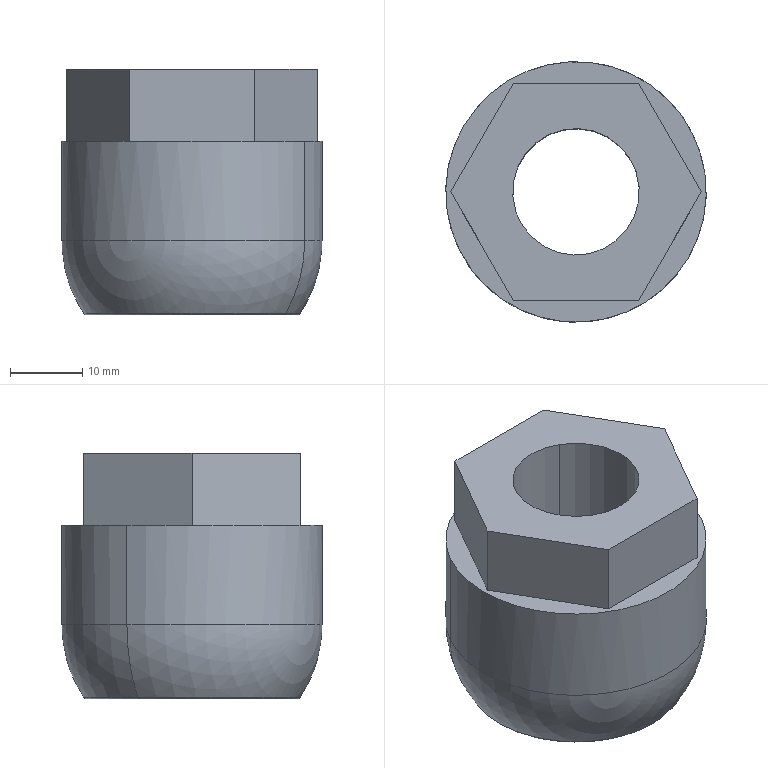CAM job | NX | 3-axis milling | part box 36 x 36 x 34 mm | stock box 36 x 36 x 34 mm
Tools:
number,name,description,diameter,corner_radius,flute_length,length,flutes
6,D6C,Milling Tool-5 Parameters,6.0,0.0,50.0,75.0,2
8,D6JING,Milling Tool-5 Parameters,6.0,0.0,50.0,75.0,2
7,D6A45,Milling Tool-5 Parameters,6.0,0.0,50.0,75.0,2
Operations:
program,operation,operation_type,tool,method,geometry_group,spindle_rpm,surface_speed,feed_per_tooth,feed_cut,feed_plunge,cut_length_mm,path_length_mm,cut_time_min,machine_time_min
1,ZLEVEL_PROFILE,ZLevelMilling,D6C,METHOD,A,4000.0,75.0,0.225,1800.0,100.0,24477.712,24544.662,13.599,13.605
1,ZLEVEL_PROFILE_COPY,ZLevelMilling,D6JING,METHOD,A,7500.0,141.0,0.0667,1000.0,100.0,128.973,205.973,0.129,0.1367
1,PLANAR_MILL,PlanarMilling,D6A45,METHOD,A,7500.0,141.0,0.0833,1250.0,100.0,116.221,175.221,0.093,0.0989